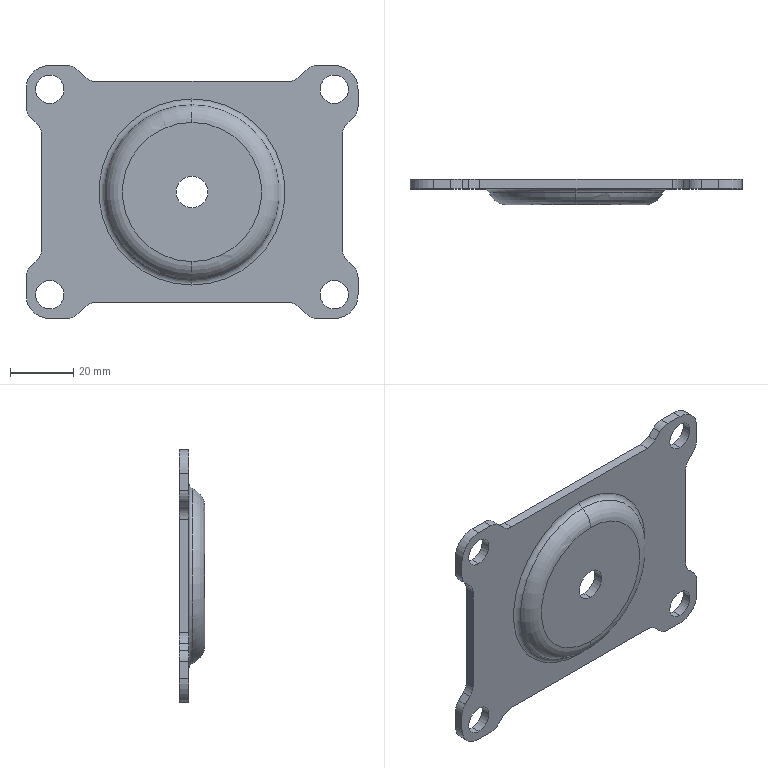Part | SolidWorks | features ICE 3, CornerTrim 2, MirrorPattern 2, FlatPattern 1, FormToolInstance 1, HoleWzd 1, SMBaseFlange 1, SheetMetal 1 | 1 solid | 62 faces | box 105 x 8 x 80 mm | volume 21623 mm3 | cylinder 30 | plane 24 | torus 8 | commonest cylinder face diameters 10 x18 9 x8 15 x4